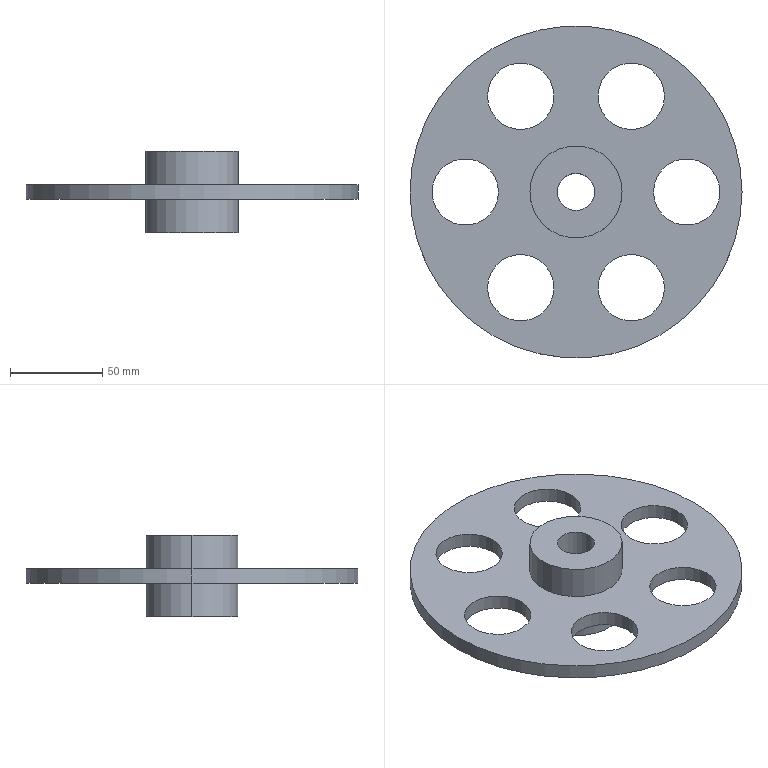Part | SolidWorks | features ICE 2, Extrusion 1 | 1 solid | 24 faces | box 180 x 180 x 44 mm | volume 211302 mm3 | cylinder 20 | plane 4 | commonest cylinder face diameters 36 x12 50 x4 20.2 x2 180 x2
STEP:
#1=CARTESIAN_POINT('',(12.,51.962,-4.));
#2=VERTEX_POINT('',#1);
#3=CARTESIAN_POINT('',(48.,51.962,-4.));
#4=VERTEX_POINT('',#3);
#5=CARTESIAN_POINT('',(30.,51.962,-4.));
#6=DIRECTION('',(0.,0.,1.));
#7=DIRECTION('',(1.,0.,0.));
#8=AXIS2_PLACEMENT_3D('',#5,#6,#7);
#9=CIRCLE('',#8,18.);
#10=EDGE_CURVE('',#2,#4,#9,.T.);
#11=ORIENTED_EDGE('',*,*,#10,.F.);
#12=CARTESIAN_POINT('',(12.,51.962,4.));
#13=VERTEX_POINT('',#12);
#14=CARTESIAN_POINT('',(12.,51.962,-30.));
#15=DIRECTION('',(0.,0.,1.));
#16=VECTOR('',#15,1000.);
#17=LINE('',#14,#16);
#18=EDGE_CURVE('',#2,#13,#17,.T.);
#19=ORIENTED_EDGE('',*,*,#18,.T.);
#20=CARTESIAN_POINT('',(48.,51.962,4.));
#21=VERTEX_POINT('',#20);
#22=CARTESIAN_POINT('',(30.,51.962,4.));
#23=DIRECTION('',(0.,0.,1.));
#24=DIRECTION('',(1.,0.,0.));
#25=AXIS2_PLACEMENT_3D('',#22,#23,#24);
#26=CIRCLE('',#25,18.);
#27=EDGE_CURVE('',#13,#21,#26,.T.);
#28=ORIENTED_EDGE('',*,*,#27,.T.);
#29=CARTESIAN_POINT('',(48.,51.962,-30.));
#30=DIRECTION('',(0.,0.,1.));
#31=VECTOR('',#30,1000.);
#32=LINE('',#29,#31);
#33=EDGE_CURVE('',#4,#21,#32,.T.);
#34=ORIENTED_EDGE('',*,*,#33,.F.);
#35=EDGE_LOOP('',(#11,#19,#28,#34));
#36=FACE_OUTER_BOUND('',#35,.T.);
#37=CARTESIAN_POINT('',(30.,51.962,-30.));
#38=DIRECTION('',(0.,0.,1.));
#39=DIRECTION('',(1.,0.,0.));
#40=AXIS2_PLACEMENT_3D('',#37,#38,#39);
#41=CYLINDRICAL_SURFACE('',#40,18.);
#42=ADVANCED_FACE('',(#36),#41,.F.);
#43=CARTESIAN_POINT('',(-48.,51.962,-4.));
#44=VERTEX_POINT('',#43);
#45=CARTESIAN_POINT('',(-12.,51.962,-4.));
#46=VERTEX_POINT('',#45);
#47=CARTESIAN_POINT('',(-30.,51.962,-4.));
#48=DIRECTION('',(0.,0.,1.));
#49=DIRECTION('',(1.,0.,0.));
#50=AXIS2_PLACEMENT_3D('',#47,#48,#49);
#51=CIRCLE('',#50,18.);
#52=EDGE_CURVE('',#44,#46,#51,.T.);
#53=ORIENTED_EDGE('',*,*,#52,.F.);
#54=CARTESIAN_POINT('',(-48.,51.962,4.));
#55=VERTEX_POINT('',#54);
#56=CARTESIAN_POINT('',(-48.,51.962,-30.));
#57=DIRECTION('',(0.,0.,1.));
#58=VECTOR('',#57,1000.);
#59=LINE('',#56,#58);
#60=EDGE_CURVE('',#44,#55,#59,.T.);
#61=ORIENTED_EDGE('',*,*,#60,.T.);
#62=CARTESIAN_POINT('',(-12.,51.962,4.));
#63=VERTEX_POINT('',#62);
#64=CARTESIAN_POINT('',(-30.,51.962,4.));
#65=DIRECTION('',(0.,0.,1.));
#66=DIRECTION('',(1.,0.,0.));
#67=AXIS2_PLACEMENT_3D('',#64,#65,#66);
#68=CIRCLE('',#67,18.);
#69=EDGE_CURVE('',#55,#63,#68,.T.);
#70=ORIENTED_EDGE('',*,*,#69,.T.);
#71=CARTESIAN_POINT('',(-12.,51.962,-30.));
#72=DIRECTION('',(0.,0.,1.));
#73=VECTOR('',#72,1000.);
#74=LINE('',#71,#73);
#75=EDGE_CURVE('',#46,#63,#74,.T.);
#76=ORIENTED_EDGE('',*,*,#75,.F.);
#77=EDGE_LOOP('',(#53,#61,#70,#76));
#78=FACE_OUTER_BOUND('',#77,.T.);
#79=CARTESIAN_POINT('',(-30.,51.962,-30.));
#80=DIRECTION('',(0.,0.,1.));
#81=DIRECTION('',(1.,0.,0.));
#82=AXIS2_PLACEMENT_3D('',#79,#80,#81);
#83=CYLINDRICAL_SURFACE('',#82,18.);
#84=ADVANCED_FACE('',(#78),#83,.F.);
#85=CARTESIAN_POINT('',(-78.,0.,-4.));
#86=VERTEX_POINT('',#85);
#87=CARTESIAN_POINT('',(-42.,0.,-4.));
#88=VERTEX_POINT('',#87);
#89=CARTESIAN_POINT('',(-60.,0.,-4.));
#90=DIRECTION('',(0.,0.,1.));
#91=DIRECTION('',(1.,0.,0.));
#92=AXIS2_PLACEMENT_3D('',#89,#90,#91);
#93=CIRCLE('',#92,18.);
#94=EDGE_CURVE('',#86,#88,#93,.T.);
#95=ORIENTED_EDGE('',*,*,#94,.F.);
#96=CARTESIAN_POINT('',(-78.,0.,4.));
#97=VERTEX_POINT('',#96);
#98=CARTESIAN_POINT('',(-78.,0.,-30.));
#99=DIRECTION('',(0.,0.,1.));
#100=VECTOR('',#99,1000.);
#101=LINE('',#98,#100);
#102=EDGE_CURVE('',#86,#97,#101,.T.);
#103=ORIENTED_EDGE('',*,*,#102,.T.);
#104=CARTESIAN_POINT('',(-42.,0.,4.));
#105=VERTEX_POINT('',#104);
#106=CARTESIAN_POINT('',(-60.,0.,4.));
#107=DIRECTION('',(0.,0.,1.));
#108=DIRECTION('',(1.,0.,0.));
#109=AXIS2_PLACEMENT_3D('',#106,#107,#108);
#110=CIRCLE('',#109,18.);
#111=EDGE_CURVE('',#97,#105,#110,.T.);
#112=ORIENTED_EDGE('',*,*,#111,.T.);
#113=CARTESIAN_POINT('',(-42.,0.,-30.));
#114=DIRECTION('',(0.,0.,1.));
#115=VECTOR('',#114,1000.);
#116=LINE('',#113,#115);
#117=EDGE_CURVE('',#88,#105,#116,.T.);
#118=ORIENTED_EDGE('',*,*,#117,.F.);
#119=EDGE_LOOP('',(#95,#103,#112,#118));
#120=FACE_OUTER_BOUND('',#119,.T.);
#121=CARTESIAN_POINT('',(-60.,0.,-30.));
#122=DIRECTION('',(0.,0.,1.));
#123=DIRECTION('',(1.,0.,0.));
#124=AXIS2_PLACEMENT_3D('',#121,#122,#123);
#125=CYLINDRICAL_SURFACE('',#124,18.);
#126=ADVANCED_FACE('',(#120),#125,.F.);
#127=CARTESIAN_POINT('',(-48.,-51.962,-4.));
#128=VERTEX_POINT('',#127);
#129=CARTESIAN_POINT('',(-12.,-51.962,-4.));
#130=VERTEX_POINT('',#129);
#131=CARTESIAN_POINT('',(-30.,-51.962,-4.));
#132=DIRECTION('',(0.,0.,1.));
#133=DIRECTION('',(1.,0.,0.));
#134=AXIS2_PLACEMENT_3D('',#131,#132,#133);
#135=CIRCLE('',#134,18.);
#136=EDGE_CURVE('',#128,#130,#135,.T.);
#137=ORIENTED_EDGE('',*,*,#136,.F.);
#138=CARTESIAN_POINT('',(-48.,-51.962,4.));
#139=VERTEX_POINT('',#138);
#140=CARTESIAN_POINT('',(-48.,-51.962,-30.));
#141=DIRECTION('',(0.,0.,1.));
#142=VECTOR('',#141,1000.);
#143=LINE('',#140,#142);
#144=EDGE_CURVE('',#128,#139,#143,.T.);
#145=ORIENTED_EDGE('',*,*,#144,.T.);
#146=CARTESIAN_POINT('',(-12.,-51.962,4.));
#147=VERTEX_POINT('',#146);
#148=CARTESIAN_POINT('',(-30.,-51.962,4.));
#149=DIRECTION('',(0.,0.,1.));
#150=DIRECTION('',(1.,0.,0.));
#151=AXIS2_PLACEMENT_3D('',#148,#149,#150);
#152=CIRCLE('',#151,18.);
#153=EDGE_CURVE('',#139,#147,#152,.T.);
#154=ORIENTED_EDGE('',*,*,#153,.T.);
#155=CARTESIAN_POINT('',(-12.,-51.962,-30.));
#156=DIRECTION('',(0.,0.,1.));
#157=VECTOR('',#156,1000.);
#158=LINE('',#155,#157);
#159=EDGE_CURVE('',#130,#147,#158,.T.);
#160=ORIENTED_EDGE('',*,*,#159,.F.);
#161=EDGE_LOOP('',(#137,#145,#154,#160));
#162=FACE_OUTER_BOUND('',#161,.T.);
#163=CARTESIAN_POINT('',(-30.,-51.962,-30.));
#164=DIRECTION('',(0.,0.,1.));
#165=DIRECTION('',(1.,0.,0.));
#166=AXIS2_PLACEMENT_3D('',#163,#164,#165);
#167=CYLINDRICAL_SURFACE('',#166,18.);
#168=ADVANCED_FACE('',(#162),#167,.F.);
#169=CARTESIAN_POINT('',(12.,-51.962,-4.));
#170=VERTEX_POINT('',#169);
#171=CARTESIAN_POINT('',(48.,-51.962,-4.));
#172=VERTEX_POINT('',#171);
#173=CARTESIAN_POINT('',(30.,-51.962,-4.));
#174=DIRECTION('',(0.,0.,1.));
#175=DIRECTION('',(1.,0.,0.));
#176=AXIS2_PLACEMENT_3D('',#173,#174,#175);
#177=CIRCLE('',#176,18.);
#178=EDGE_CURVE('',#170,#172,#177,.T.);
#179=ORIENTED_EDGE('',*,*,#178,.F.);
#180=CARTESIAN_POINT('',(12.,-51.962,4.));
#181=VERTEX_POINT('',#180);
#182=CARTESIAN_POINT('',(12.,-51.962,-30.));
#183=DIRECTION('',(0.,0.,1.));
#184=VECTOR('',#183,1000.);
#185=LINE('',#182,#184);
#186=EDGE_CURVE('',#170,#181,#185,.T.);
#187=ORIENTED_EDGE('',*,*,#186,.T.);
#188=CARTESIAN_POINT('',(48.,-51.962,4.));
#189=VERTEX_POINT('',#188);
#190=CARTESIAN_POINT('',(30.,-51.962,4.));
#191=DIRECTION('',(0.,0.,1.));
#192=DIRECTION('',(1.,0.,0.));
#193=AXIS2_PLACEMENT_3D('',#190,#191,#192);
#194=CIRCLE('',#193,18.);
#195=EDGE_CURVE('',#181,#189,#194,.T.);
#196=ORIENTED_EDGE('',*,*,#195,.T.);
#197=CARTESIAN_POINT('',(48.,-51.962,-30.));
#198=DIRECTION('',(0.,0.,1.));
#199=VECTOR('',#198,1000.);
#200=LINE('',#197,#199);
#201=EDGE_CURVE('',#172,#189,#200,.T.);
#202=ORIENTED_EDGE('',*,*,#201,.F.);
#203=EDGE_LOOP('',(#179,#187,#196,#202));
#204=FACE_OUTER_BOUND('',#203,.T.);
#205=CARTESIAN_POINT('',(30.,-51.962,-30.));
#206=DIRECTION('',(0.,0.,1.));
#207=DIRECTION('',(1.,0.,0.));
#208=AXIS2_PLACEMENT_3D('',#205,#206,#207);
#209=CYLINDRICAL_SURFACE('',#208,18.);
#210=ADVANCED_FACE('',(#204),#209,.F.);
#211=CARTESIAN_POINT('',(42.,0.,-4.));
#212=VERTEX_POINT('',#211);
#213=CARTESIAN_POINT('',(78.,0.,-4.));
#214=VERTEX_POINT('',#213);
#215=CARTESIAN_POINT('',(60.,0.,-4.));
#216=DIRECTION('',(0.,0.,1.));
#217=DIRECTION('',(1.,0.,0.));
#218=AXIS2_PLACEMENT_3D('',#215,#216,#217);
#219=CIRCLE('',#218,18.);
#220=EDGE_CURVE('',#212,#214,#219,.T.);
#221=ORIENTED_EDGE('',*,*,#220,.F.);
#222=CARTESIAN_POINT('',(42.,0.,4.));
#223=VERTEX_POINT('',#222);
#224=CARTESIAN_POINT('',(42.,0.,-30.));
#225=DIRECTION('',(0.,0.,1.));
#226=VECTOR('',#225,1000.);
#227=LINE('',#224,#226);
#228=EDGE_CURVE('',#212,#223,#227,.T.);
#229=ORIENTED_EDGE('',*,*,#228,.T.);
#230=CARTESIAN_POINT('',(78.,0.,4.));
#231=VERTEX_POINT('',#230);
#232=CARTESIAN_POINT('',(60.,0.,4.));
#233=DIRECTION('',(0.,0.,1.));
#234=DIRECTION('',(1.,0.,0.));
#235=AXIS2_PLACEMENT_3D('',#232,#233,#234);
#236=CIRCLE('',#235,18.);
#237=EDGE_CURVE('',#223,#231,#236,.T.);
#238=ORIENTED_EDGE('',*,*,#237,.T.);
#239=CARTESIAN_POINT('',(78.,0.,-30.));
#240=DIRECTION('',(0.,0.,1.));
#241=VECTOR('',#240,1000.);
#242=LINE('',#239,#241);
#243=EDGE_CURVE('',#214,#231,#242,.T.);
#244=ORIENTED_EDGE('',*,*,#243,.F.);
#245=EDGE_LOOP('',(#221,#229,#238,#244));
#246=FACE_OUTER_BOUND('',#245,.T.);
#247=CARTESIAN_POINT('',(60.,0.,-30.));
#248=DIRECTION('',(0.,0.,1.));
#249=DIRECTION('',(1.,0.,0.));
#250=AXIS2_PLACEMENT_3D('',#247,#248,#249);
#251=CYLINDRICAL_SURFACE('',#250,18.);
#252=ADVANCED_FACE('',(#246),#251,.F.);
#253=CARTESIAN_POINT('',(-10.1,0.,-22.));
#254=VERTEX_POINT('',#253);
#255=CARTESIAN_POINT('',(10.1,0.,-22.));
#256=VERTEX_POINT('',#255);
#257=CARTESIAN_POINT('',(0.,0.,-22.));
#258=DIRECTION('',(0.,0.,1.));
#259=DIRECTION('',(1.,0.,0.));
#260=AXIS2_PLACEMENT_3D('',#257,#258,#259);
#261=CIRCLE('',#260,10.1);
#262=EDGE_CURVE('',#254,#256,#261,.T.);
#263=ORIENTED_EDGE('',*,*,#262,.F.);
#264=CARTESIAN_POINT('',(-10.1,0.,22.));
#265=VERTEX_POINT('',#264);
#266=CARTESIAN_POINT('',(-10.1,0.,-4.));
#267=DIRECTION('',(0.,0.,1.));
#268=VECTOR('',#267,1000.);
#269=LINE('',#266,#268);
#270=EDGE_CURVE('',#254,#265,#269,.T.);
#271=ORIENTED_EDGE('',*,*,#270,.T.);
#272=CARTESIAN_POINT('',(10.1,0.,22.));
#273=VERTEX_POINT('',#272);
#274=CARTESIAN_POINT('',(0.,0.,22.));
#275=DIRECTION('',(0.,0.,1.));
#276=DIRECTION('',(1.,0.,0.));
#277=AXIS2_PLACEMENT_3D('',#274,#275,#276);
#278=CIRCLE('',#277,10.1);
#279=EDGE_CURVE('',#265,#273,#278,.T.);
#280=ORIENTED_EDGE('',*,*,#279,.T.);
#281=CARTESIAN_POINT('',(10.1,0.,-4.));
#282=DIRECTION('',(0.,0.,1.));
#283=VECTOR('',#282,1000.);
#284=LINE('',#281,#283);
#285=EDGE_CURVE('',#256,#273,#284,.T.);
#286=ORIENTED_EDGE('',*,*,#285,.F.);
#287=EDGE_LOOP('',(#263,#271,#280,#286));
#288=FACE_OUTER_BOUND('',#287,.T.);
#289=CARTESIAN_POINT('',(0.,0.,-4.));
#290=DIRECTION('',(0.,0.,1.));
#291=DIRECTION('',(1.,0.,0.));
#292=AXIS2_PLACEMENT_3D('',#289,#290,#291);
#293=CYLINDRICAL_SURFACE('',#292,10.1);
#294=ADVANCED_FACE('',(#288),#293,.F.);
#295=CARTESIAN_POINT('',(25.,0.,-22.));
#296=VERTEX_POINT('',#295);
#297=CARTESIAN_POINT('',(-25.,0.,-22.));
#298=VERTEX_POINT('',#297);
#299=CARTESIAN_POINT('',(0.,0.,-22.));
#300=DIRECTION('',(0.,0.,1.));
#301=DIRECTION('',(1.,0.,0.));
#302=AXIS2_PLACEMENT_3D('',#299,#300,#301);
#303=CIRCLE('',#302,25.);
#304=EDGE_CURVE('',#296,#298,#303,.T.);
#305=ORIENTED_EDGE('',*,*,#304,.T.);
#306=CARTESIAN_POINT('',(-25.,0.,-4.));
#307=VERTEX_POINT('',#306);
#308=CARTESIAN_POINT('',(-25.,0.,-22.));
#309=DIRECTION('',(0.,0.,1.));
#310=VECTOR('',#309,1000.);
#311=LINE('',#308,#310);
#312=EDGE_CURVE('',#298,#307,#311,.T.);
#313=ORIENTED_EDGE('',*,*,#312,.T.);
#314=CARTESIAN_POINT('',(25.,0.,-4.));
#315=VERTEX_POINT('',#314);
#316=CARTESIAN_POINT('',(0.,0.,-4.));
#317=DIRECTION('',(0.,0.,1.));
#318=DIRECTION('',(1.,0.,0.));
#319=AXIS2_PLACEMENT_3D('',#316,#317,#318);
#320=CIRCLE('',#319,25.);
#321=EDGE_CURVE('',#315,#307,#320,.T.);
#322=ORIENTED_EDGE('',*,*,#321,.F.);
#323=CARTESIAN_POINT('',(25.,0.,-22.));
#324=DIRECTION('',(0.,0.,1.));
#325=VECTOR('',#324,1000.);
#326=LINE('',#323,#325);
#327=EDGE_CURVE('',#296,#315,#326,.T.);
#328=ORIENTED_EDGE('',*,*,#327,.F.);
#329=EDGE_LOOP('',(#305,#313,#322,#328));
#330=FACE_OUTER_BOUND('',#329,.T.);
#331=CARTESIAN_POINT('',(0.,0.,-22.));
#332=DIRECTION('',(0.,0.,1.));
#333=DIRECTION('',(1.,0.,0.));
#334=AXIS2_PLACEMENT_3D('',#331,#332,#333);
#335=CYLINDRICAL_SURFACE('',#334,25.);
#336=ADVANCED_FACE('',(#330),#335,.T.);
#337=CARTESIAN_POINT('',(25.,0.,4.));
#338=VERTEX_POINT('',#337);
#339=CARTESIAN_POINT('',(-25.,0.,4.));
#340=VERTEX_POINT('',#339);
#341=CARTESIAN_POINT('',(0.,0.,4.));
#342=DIRECTION('',(0.,0.,1.));
#343=DIRECTION('',(1.,0.,0.));
#344=AXIS2_PLACEMENT_3D('',#341,#342,#343);
#345=CIRCLE('',#344,25.);
#346=EDGE_CURVE('',#338,#340,#345,.T.);
#347=ORIENTED_EDGE('',*,*,#346,.T.);
#348=CARTESIAN_POINT('',(-25.,0.,22.));
#349=VERTEX_POINT('',#348);
#350=CARTESIAN_POINT('',(-25.,0.,-22.));
#351=DIRECTION('',(0.,0.,1.));
#352=VECTOR('',#351,1000.);
#353=LINE('',#350,#352);
#354=EDGE_CURVE('',#340,#349,#353,.T.);
#355=ORIENTED_EDGE('',*,*,#354,.T.);
#356=CARTESIAN_POINT('',(25.,0.,22.));
#357=VERTEX_POINT('',#356);
#358=CARTESIAN_POINT('',(0.,0.,22.));
#359=DIRECTION('',(0.,0.,1.));
#360=DIRECTION('',(1.,0.,0.));
#361=AXIS2_PLACEMENT_3D('',#358,#359,#360);
#362=CIRCLE('',#361,25.);
#363=EDGE_CURVE('',#357,#349,#362,.T.);
#364=ORIENTED_EDGE('',*,*,#363,.F.);
#365=CARTESIAN_POINT('',(25.,0.,-22.));
#366=DIRECTION('',(0.,0.,1.));
#367=VECTOR('',#366,1000.);
#368=LINE('',#365,#367);
#369=EDGE_CURVE('',#338,#357,#368,.T.);
#370=ORIENTED_EDGE('',*,*,#369,.F.);
#371=EDGE_LOOP('',(#347,#355,#364,#370));
#372=FACE_OUTER_BOUND('',#371,.T.);
#373=CARTESIAN_POINT('',(0.,0.,-22.));
#374=DIRECTION('',(0.,0.,1.));
#375=DIRECTION('',(1.,0.,0.));
#376=AXIS2_PLACEMENT_3D('',#373,#374,#375);
#377=CYLINDRICAL_SURFACE('',#376,25.);
#378=ADVANCED_FACE('',(#372),#377,.T.);
#379=CARTESIAN_POINT('',(90.,0.,-4.));
#380=VERTEX_POINT('',#379);
#381=CARTESIAN_POINT('',(-90.,0.,-4.));
#382=VERTEX_POINT('',#381);
#383=CARTESIAN_POINT('',(0.,0.,-4.));
#384=DIRECTION('',(0.,0.,1.));
#385=DIRECTION('',(1.,0.,0.));
#386=AXIS2_PLACEMENT_3D('',#383,#384,#385);
#387=CIRCLE('',#386,90.);
#388=EDGE_CURVE('',#380,#382,#387,.T.);
#389=ORIENTED_EDGE('',*,*,#388,.T.);
#390=CARTESIAN_POINT('',(-90.,0.,4.));
#391=VERTEX_POINT('',#390);
#392=CARTESIAN_POINT('',(-90.,0.,-4.));
#393=DIRECTION('',(0.,0.,1.));
#394=VECTOR('',#393,1000.);
#395=LINE('',#392,#394);
#396=EDGE_CURVE('',#382,#391,#395,.T.);
#397=ORIENTED_EDGE('',*,*,#396,.T.);
#398=CARTESIAN_POINT('',(90.,0.,4.));
#399=VERTEX_POINT('',#398);
#400=CARTESIAN_POINT('',(0.,0.,4.));
#401=DIRECTION('',(0.,0.,1.));
#402=DIRECTION('',(1.,0.,0.));
#403=AXIS2_PLACEMENT_3D('',#400,#401,#402);
#404=CIRCLE('',#403,90.);
#405=EDGE_CURVE('',#399,#391,#404,.T.);
#406=ORIENTED_EDGE('',*,*,#405,.F.);
#407=CARTESIAN_POINT('',(90.,0.,-4.));
#408=DIRECTION('',(0.,0.,1.));
#409=VECTOR('',#408,1000.);
#410=LINE('',#407,#409);
#411=EDGE_CURVE('',#380,#399,#410,.T.);
#412=ORIENTED_EDGE('',*,*,#411,.F.);
#413=EDGE_LOOP('',(#389,#397,#406,#412));
#414=FACE_OUTER_BOUND('',#413,.T.);
#415=CARTESIAN_POINT('',(0.,0.,-4.));
#416=DIRECTION('',(0.,0.,1.));
#417=DIRECTION('',(1.,0.,0.));
#418=AXIS2_PLACEMENT_3D('',#415,#416,#417);
#419=CYLINDRICAL_SURFACE('',#418,90.);
#420=ADVANCED_FACE('',(#414),#419,.T.);
#421=ORIENTED_EDGE('',*,*,#396,.F.);
#422=CARTESIAN_POINT('',(0.,0.,-4.));
#423=DIRECTION('',(0.,0.,1.));
#424=DIRECTION('',(1.,0.,0.));
#425=AXIS2_PLACEMENT_3D('',#422,#423,#424);
#426=CIRCLE('',#425,90.);
#427=EDGE_CURVE('',#382,#380,#426,.T.);
#428=ORIENTED_EDGE('',*,*,#427,.T.);
#429=ORIENTED_EDGE('',*,*,#411,.T.);
#430=CARTESIAN_POINT('',(0.,0.,4.));
#431=DIRECTION('',(0.,0.,1.));
#432=DIRECTION('',(1.,0.,0.));
#433=AXIS2_PLACEMENT_3D('',#430,#431,#432);
#434=CIRCLE('',#433,90.);
#435=EDGE_CURVE('',#391,#399,#434,.T.);
#436=ORIENTED_EDGE('',*,*,#435,.F.);
#437=EDGE_LOOP('',(#421,#428,#429,#436));
#438=FACE_OUTER_BOUND('',#437,.T.);
#439=CARTESIAN_POINT('',(0.,0.,-4.));
#440=DIRECTION('',(0.,0.,1.));
#441=DIRECTION('',(1.,0.,0.));
#442=AXIS2_PLACEMENT_3D('',#439,#440,#441);
#443=CYLINDRICAL_SURFACE('',#442,90.);
#444=ADVANCED_FACE('',(#438),#443,.T.);
#445=CARTESIAN_POINT('',(30.,51.962,-4.));
#446=DIRECTION('',(0.,0.,1.));
#447=DIRECTION('',(1.,0.,0.));
#448=AXIS2_PLACEMENT_3D('',#445,#446,#447);
#449=CIRCLE('',#448,18.);
#450=EDGE_CURVE('',#4,#2,#449,.T.);
#451=ORIENTED_EDGE('',*,*,#450,.T.);
#452=ORIENTED_EDGE('',*,*,#10,.T.);
#453=EDGE_LOOP('',(#451,#452));
#454=FACE_BOUND('',#453,.T.);
#455=CARTESIAN_POINT('',(-30.,51.962,-4.));
#456=DIRECTION('',(0.,0.,1.));
#457=DIRECTION('',(1.,0.,0.));
#458=AXIS2_PLACEMENT_3D('',#455,#456,#457);
#459=CIRCLE('',#458,18.);
#460=EDGE_CURVE('',#46,#44,#459,.T.);
#461=ORIENTED_EDGE('',*,*,#460,.T.);
#462=ORIENTED_EDGE('',*,*,#52,.T.);
#463=EDGE_LOOP('',(#461,#462));
#464=FACE_BOUND('',#463,.T.);
#465=CARTESIAN_POINT('',(-60.,0.,-4.));
#466=DIRECTION('',(0.,0.,1.));
#467=DIRECTION('',(1.,0.,0.));
#468=AXIS2_PLACEMENT_3D('',#465,#466,#467);
#469=CIRCLE('',#468,18.);
#470=EDGE_CURVE('',#88,#86,#469,.T.);
#471=ORIENTED_EDGE('',*,*,#470,.T.);
#472=ORIENTED_EDGE('',*,*,#94,.T.);
#473=EDGE_LOOP('',(#471,#472));
#474=FACE_BOUND('',#473,.T.);
#475=CARTESIAN_POINT('',(-30.,-51.962,-4.));
#476=DIRECTION('',(0.,0.,1.));
#477=DIRECTION('',(1.,0.,0.));
#478=AXIS2_PLACEMENT_3D('',#475,#476,#477);
#479=CIRCLE('',#478,18.);
#480=EDGE_CURVE('',#130,#128,#479,.T.);
#481=ORIENTED_EDGE('',*,*,#480,.T.);
#482=ORIENTED_EDGE('',*,*,#136,.T.);
#483=EDGE_LOOP('',(#481,#482));
#484=FACE_BOUND('',#483,.T.);
#485=CARTESIAN_POINT('',(30.,-51.962,-4.));
#486=DIRECTION('',(0.,0.,1.));
#487=DIRECTION('',(1.,0.,0.));
#488=AXIS2_PLACEMENT_3D('',#485,#486,#487);
#489=CIRCLE('',#488,18.);
#490=EDGE_CURVE('',#172,#170,#489,.T.);
#491=ORIENTED_EDGE('',*,*,#490,.T.);
#492=ORIENTED_EDGE('',*,*,#178,.T.);
#493=EDGE_LOOP('',(#491,#492));
#494=FACE_BOUND('',#493,.T.);
#495=CARTESIAN_POINT('',(60.,0.,-4.));
#496=DIRECTION('',(0.,0.,1.));
#497=DIRECTION('',(1.,0.,0.));
#498=AXIS2_PLACEMENT_3D('',#495,#496,#497);
#499=CIRCLE('',#498,18.);
#500=EDGE_CURVE('',#214,#212,#499,.T.);
#501=ORIENTED_EDGE('',*,*,#500,.T.);
#502=ORIENTED_EDGE('',*,*,#220,.T.);
#503=EDGE_LOOP('',(#501,#502));
#504=FACE_BOUND('',#503,.T.);
#505=ORIENTED_EDGE('',*,*,#321,.T.);
#506=CARTESIAN_POINT('',(0.,0.,-4.));
#507=DIRECTION('',(0.,0.,1.));
#508=DIRECTION('',(1.,0.,0.));
#509=AXIS2_PLACEMENT_3D('',#506,#507,#508);
#510=CIRCLE('',#509,25.);
#511=EDGE_CURVE('',#307,#315,#510,.T.);
#512=ORIENTED_EDGE('',*,*,#511,.T.);
#513=EDGE_LOOP('',(#505,#512));
#514=FACE_BOUND('',#513,.T.);
#515=ORIENTED_EDGE('',*,*,#388,.F.);
#516=ORIENTED_EDGE('',*,*,#427,.F.);
#517=EDGE_LOOP('',(#515,#516));
#518=FACE_OUTER_BOUND('',#517,.T.);
#519=CARTESIAN_POINT('',(0.,0.,-4.));
#520=DIRECTION('',(0.,0.,1.));
#521=DIRECTION('',(1.,0.,0.));
#522=AXIS2_PLACEMENT_3D('',#519,#520,#521);
#523=PLANE('',#522);
#524=ADVANCED_FACE('',(#454,#464,#474,#484,#494,#504,#514,#518),#523,.F.);
#525=CARTESIAN_POINT('',(30.,51.962,4.));
#526=DIRECTION('',(0.,0.,1.));
#527=DIRECTION('',(1.,0.,0.));
#528=AXIS2_PLACEMENT_3D('',#525,#526,#527);
#529=CIRCLE('',#528,18.);
#530=EDGE_CURVE('',#21,#13,#529,.T.);
#531=ORIENTED_EDGE('',*,*,#530,.F.);
#532=ORIENTED_EDGE('',*,*,#27,.F.);
#533=EDGE_LOOP('',(#531,#532));
#534=FACE_BOUND('',#533,.T.);
#535=CARTESIAN_POINT('',(-30.,51.962,4.));
#536=DIRECTION('',(0.,0.,1.));
#537=DIRECTION('',(1.,0.,0.));
#538=AXIS2_PLACEMENT_3D('',#535,#536,#537);
#539=CIRCLE('',#538,18.);
#540=EDGE_CURVE('',#63,#55,#539,.T.);
#541=ORIENTED_EDGE('',*,*,#540,.F.);
#542=ORIENTED_EDGE('',*,*,#69,.F.);
#543=EDGE_LOOP('',(#541,#542));
#544=FACE_BOUND('',#543,.T.);
#545=CARTESIAN_POINT('',(-60.,0.,4.));
#546=DIRECTION('',(0.,0.,1.));
#547=DIRECTION('',(1.,0.,0.));
#548=AXIS2_PLACEMENT_3D('',#545,#546,#547);
#549=CIRCLE('',#548,18.);
#550=EDGE_CURVE('',#105,#97,#549,.T.);
#551=ORIENTED_EDGE('',*,*,#550,.F.);
#552=ORIENTED_EDGE('',*,*,#111,.F.);
#553=EDGE_LOOP('',(#551,#552));
#554=FACE_BOUND('',#553,.T.);
#555=CARTESIAN_POINT('',(-30.,-51.962,4.));
#556=DIRECTION('',(0.,0.,1.));
#557=DIRECTION('',(1.,0.,0.));
#558=AXIS2_PLACEMENT_3D('',#555,#556,#557);
#559=CIRCLE('',#558,18.);
#560=EDGE_CURVE('',#147,#139,#559,.T.);
#561=ORIENTED_EDGE('',*,*,#560,.F.);
#562=ORIENTED_EDGE('',*,*,#153,.F.);
#563=EDGE_LOOP('',(#561,#562));
#564=FACE_BOUND('',#563,.T.);
#565=CARTESIAN_POINT('',(30.,-51.962,4.));
#566=DIRECTION('',(0.,0.,1.));
#567=DIRECTION('',(1.,0.,0.));
#568=AXIS2_PLACEMENT_3D('',#565,#566,#567);
#569=CIRCLE('',#568,18.);
#570=EDGE_CURVE('',#189,#181,#569,.T.);
#571=ORIENTED_EDGE('',*,*,#570,.F.);
#572=ORIENTED_EDGE('',*,*,#195,.F.);
#573=EDGE_LOOP('',(#571,#572));
#574=FACE_BOUND('',#573,.T.);
#575=CARTESIAN_POINT('',(60.,0.,4.));
#576=DIRECTION('',(0.,0.,1.));
#577=DIRECTION('',(1.,0.,0.));
#578=AXIS2_PLACEMENT_3D('',#575,#576,#577);
#579=CIRCLE('',#578,18.);
#580=EDGE_CURVE('',#231,#223,#579,.T.);
#581=ORIENTED_EDGE('',*,*,#580,.F.);
#582=ORIENTED_EDGE('',*,*,#237,.F.);
#583=EDGE_LOOP('',(#581,#582));
#584=FACE_BOUND('',#583,.T.);
#585=ORIENTED_EDGE('',*,*,#346,.F.);
#586=CARTESIAN_POINT('',(0.,0.,4.));
#587=DIRECTION('',(0.,0.,1.));
#588=DIRECTION('',(1.,0.,0.));
#589=AXIS2_PLACEMENT_3D('',#586,#587,#588);
#590=CIRCLE('',#589,25.);
#591=EDGE_CURVE('',#340,#338,#590,.T.);
#592=ORIENTED_EDGE('',*,*,#591,.F.);
#593=EDGE_LOOP('',(#585,#592));
#594=FACE_BOUND('',#593,.T.);
#595=ORIENTED_EDGE('',*,*,#405,.T.);
#596=ORIENTED_EDGE('',*,*,#435,.T.);
#597=EDGE_LOOP('',(#595,#596));
#598=FACE_OUTER_BOUND('',#597,.T.);
#599=CARTESIAN_POINT('',(0.,0.,4.));
#600=DIRECTION('',(0.,0.,1.));
#601=DIRECTION('',(1.,0.,0.));
#602=AXIS2_PLACEMENT_3D('',#599,#600,#601);
#603=PLANE('',#602);
#604=ADVANCED_FACE('',(#534,#544,#554,#564,#574,#584,#594,#598),#603,.T.);
#605=ORIENTED_EDGE('',*,*,#354,.F.);
#606=ORIENTED_EDGE('',*,*,#591,.T.);
#607=ORIENTED_EDGE('',*,*,#369,.T.);
#608=CARTESIAN_POINT('',(0.,0.,22.));
#609=DIRECTION('',(0.,0.,1.));
#610=DIRECTION('',(1.,0.,0.));
#611=AXIS2_PLACEMENT_3D('',#608,#609,#610);
#612=CIRCLE('',#611,25.);
#613=EDGE_CURVE('',#349,#357,#612,.T.);
#614=ORIENTED_EDGE('',*,*,#613,.F.);
#615=EDGE_LOOP('',(#605,#606,#607,#614));
#616=FACE_OUTER_BOUND('',#615,.T.);
#617=CARTESIAN_POINT('',(0.,0.,-22.));
#618=DIRECTION('',(0.,0.,1.));
#619=DIRECTION('',(1.,0.,0.));
#620=AXIS2_PLACEMENT_3D('',#617,#618,#619);
#621=CYLINDRICAL_SURFACE('',#620,25.);
#622=ADVANCED_FACE('',(#616),#621,.T.);
#623=CARTESIAN_POINT('',(0.,0.,22.));
#624=DIRECTION('',(0.,0.,1.));
#625=DIRECTION('',(1.,0.,0.));
#626=AXIS2_PLACEMENT_3D('',#623,#624,#625);
#627=CIRCLE('',#626,10.1);
#628=EDGE_CURVE('',#273,#265,#627,.T.);
#629=ORIENTED_EDGE('',*,*,#628,.F.);
#630=ORIENTED_EDGE('',*,*,#279,.F.);
#631=EDGE_LOOP('',(#629,#630));
#632=FACE_BOUND('',#631,.T.);
#633=ORIENTED_EDGE('',*,*,#363,.T.);
#634=ORIENTED_EDGE('',*,*,#613,.T.);
#635=EDGE_LOOP('',(#633,#634));
#636=FACE_OUTER_BOUND('',#635,.T.);
#637=CARTESIAN_POINT('',(0.,0.,22.));
#638=DIRECTION('',(0.,0.,1.));
#639=DIRECTION('',(1.,0.,0.));
#640=AXIS2_PLACEMENT_3D('',#637,#638,#639);
#641=PLANE('',#640);
#642=ADVANCED_FACE('',(#632,#636),#641,.T.);
#643=ORIENTED_EDGE('',*,*,#312,.F.);
#644=CARTESIAN_POINT('',(0.,0.,-22.));
#645=DIRECTION('',(0.,0.,1.));
#646=DIRECTION('',(1.,0.,0.));
#647=AXIS2_PLACEMENT_3D('',#644,#645,#646);
#648=CIRCLE('',#647,25.);
#649=EDGE_CURVE('',#298,#296,#648,.T.);
#650=ORIENTED_EDGE('',*,*,#649,.T.);
#651=ORIENTED_EDGE('',*,*,#327,.T.);
#652=ORIENTED_EDGE('',*,*,#511,.F.);
#653=EDGE_LOOP('',(#643,#650,#651,#652));
#654=FACE_OUTER_BOUND('',#653,.T.);
#655=CARTESIAN_POINT('',(0.,0.,-22.));
#656=DIRECTION('',(0.,0.,1.));
#657=DIRECTION('',(1.,0.,0.));
#658=AXIS2_PLACEMENT_3D('',#655,#656,#657);
#659=CYLINDRICAL_SURFACE('',#658,25.);
#660=ADVANCED_FACE('',(#654),#659,.T.);
#661=CARTESIAN_POINT('',(0.,0.,-22.));
#662=DIRECTION('',(0.,0.,1.));
#663=DIRECTION('',(1.,0.,0.));
#664=AXIS2_PLACEMENT_3D('',#661,#662,#663);
#665=CIRCLE('',#664,10.1);
#666=EDGE_CURVE('',#256,#254,#665,.T.);
#667=ORIENTED_EDGE('',*,*,#666,.T.);
#668=ORIENTED_EDGE('',*,*,#262,.T.);
#669=EDGE_LOOP('',(#667,#668));
#670=FACE_BOUND('',#669,.T.);
#671=ORIENTED_EDGE('',*,*,#304,.F.);
#672=ORIENTED_EDGE('',*,*,#649,.F.);
#673=EDGE_LOOP('',(#671,#672));
#674=FACE_OUTER_BOUND('',#673,.T.);
#675=CARTESIAN_POINT('',(0.,0.,-22.));
#676=DIRECTION('',(0.,0.,1.));
#677=DIRECTION('',(1.,0.,0.));
#678=AXIS2_PLACEMENT_3D('',#675,#676,#677);
#679=PLANE('',#678);
#680=ADVANCED_FACE('',(#670,#674),#679,.F.);
#681=ORIENTED_EDGE('',*,*,#270,.F.);
#682=ORIENTED_EDGE('',*,*,#666,.F.);
#683=ORIENTED_EDGE('',*,*,#285,.T.);
#684=ORIENTED_EDGE('',*,*,#628,.T.);
#685=EDGE_LOOP('',(#681,#682,#683,#684));
#686=FACE_OUTER_BOUND('',#685,.T.);
#687=CARTESIAN_POINT('',(0.,0.,-4.));
#688=DIRECTION('',(0.,0.,1.));
#689=DIRECTION('',(1.,0.,0.));
#690=AXIS2_PLACEMENT_3D('',#687,#688,#689);
#691=CYLINDRICAL_SURFACE('',#690,10.1);
#692=ADVANCED_FACE('',(#686),#691,.F.);
#693=ORIENTED_EDGE('',*,*,#228,.F.);
#694=ORIENTED_EDGE('',*,*,#500,.F.);
#695=ORIENTED_EDGE('',*,*,#243,.T.);
#696=ORIENTED_EDGE('',*,*,#580,.T.);
#697=EDGE_LOOP('',(#693,#694,#695,#696));
#698=FACE_OUTER_BOUND('',#697,.T.);
#699=CARTESIAN_POINT('',(60.,0.,-30.));
#700=DIRECTION('',(0.,0.,1.));
#701=DIRECTION('',(1.,0.,0.));
#702=AXIS2_PLACEMENT_3D('',#699,#700,#701);
#703=CYLINDRICAL_SURFACE('',#702,18.);
#704=ADVANCED_FACE('',(#698),#703,.F.);
#705=ORIENTED_EDGE('',*,*,#186,.F.);
#706=ORIENTED_EDGE('',*,*,#490,.F.);
#707=ORIENTED_EDGE('',*,*,#201,.T.);
#708=ORIENTED_EDGE('',*,*,#570,.T.);
#709=EDGE_LOOP('',(#705,#706,#707,#708));
#710=FACE_OUTER_BOUND('',#709,.T.);
#711=CARTESIAN_POINT('',(30.,-51.962,-30.));
#712=DIRECTION('',(0.,0.,1.));
#713=DIRECTION('',(1.,0.,0.));
#714=AXIS2_PLACEMENT_3D('',#711,#712,#713);
#715=CYLINDRICAL_SURFACE('',#714,18.);
#716=ADVANCED_FACE('',(#710),#715,.F.);
#717=ORIENTED_EDGE('',*,*,#144,.F.);
#718=ORIENTED_EDGE('',*,*,#480,.F.);
#719=ORIENTED_EDGE('',*,*,#159,.T.);
#720=ORIENTED_EDGE('',*,*,#560,.T.);
#721=EDGE_LOOP('',(#717,#718,#719,#720));
#722=FACE_OUTER_BOUND('',#721,.T.);
#723=CARTESIAN_POINT('',(-30.,-51.962,-30.));
#724=DIRECTION('',(0.,0.,1.));
#725=DIRECTION('',(1.,0.,0.));
#726=AXIS2_PLACEMENT_3D('',#723,#724,#725);
#727=CYLINDRICAL_SURFACE('',#726,18.);
#728=ADVANCED_FACE('',(#722),#727,.F.);
#729=ORIENTED_EDGE('',*,*,#102,.F.);
#730=ORIENTED_EDGE('',*,*,#470,.F.);
#731=ORIENTED_EDGE('',*,*,#117,.T.);
#732=ORIENTED_EDGE('',*,*,#550,.T.);
#733=EDGE_LOOP('',(#729,#730,#731,#732));
#734=FACE_OUTER_BOUND('',#733,.T.);
#735=CARTESIAN_POINT('',(-60.,0.,-30.));
#736=DIRECTION('',(0.,0.,1.));
#737=DIRECTION('',(1.,0.,0.));
#738=AXIS2_PLACEMENT_3D('',#735,#736,#737);
#739=CYLINDRICAL_SURFACE('',#738,18.);
#740=ADVANCED_FACE('',(#734),#739,.F.);
#741=ORIENTED_EDGE('',*,*,#60,.F.);
#742=ORIENTED_EDGE('',*,*,#460,.F.);
#743=ORIENTED_EDGE('',*,*,#75,.T.);
#744=ORIENTED_EDGE('',*,*,#540,.T.);
#745=EDGE_LOOP('',(#741,#742,#743,#744));
#746=FACE_OUTER_BOUND('',#745,.T.);
#747=CARTESIAN_POINT('',(-30.,51.962,-30.));
#748=DIRECTION('',(0.,0.,1.));
#749=DIRECTION('',(1.,0.,0.));
#750=AXIS2_PLACEMENT_3D('',#747,#748,#749);
#751=CYLINDRICAL_SURFACE('',#750,18.);
#752=ADVANCED_FACE('',(#746),#751,.F.);
#753=ORIENTED_EDGE('',*,*,#18,.F.);
#754=ORIENTED_EDGE('',*,*,#450,.F.);
#755=ORIENTED_EDGE('',*,*,#33,.T.);
#756=ORIENTED_EDGE('',*,*,#530,.T.);
#757=EDGE_LOOP('',(#753,#754,#755,#756));
#758=FACE_OUTER_BOUND('',#757,.T.);
#759=CARTESIAN_POINT('',(30.,51.962,-30.));
#760=DIRECTION('',(0.,0.,1.));
#761=DIRECTION('',(1.,0.,0.));
#762=AXIS2_PLACEMENT_3D('',#759,#760,#761);
#763=CYLINDRICAL_SURFACE('',#762,18.);
#764=ADVANCED_FACE('',(#758),#763,.F.);
#765=CLOSED_SHELL('',(#42,#84,#126,#168,#210,#252,#294,#336,#378,#420,#444,#524,#604,#622,#642,#660,#680,#692,#704,#716,#728,#740,#752,#764));
#766=MANIFOLD_SOLID_BREP('',#765);
#767=CARTESIAN_POINT('',(0.,0.,0.));
#768=DIRECTION('',(0.,0.,1.));
#769=DIRECTION('',(1.,0.,0.));
#770=AXIS2_PLACEMENT_3D('',#767,#768,#769);
#771=(LENGTH_UNIT()NAMED_UNIT(*)SI_UNIT(.MILLI.,.METRE.));
#772=UNCERTAINTY_MEASURE_WITH_UNIT(LENGTH_MEASURE(0.00001),#771,'','');
#773=(NAMED_UNIT(*)PLANE_ANGLE_UNIT()SI_UNIT($,.RADIAN.));
#774=(NAMED_UNIT(*)SI_UNIT($,.STERADIAN.)SOLID_ANGLE_UNIT());
#775=(GEOMETRIC_REPRESENTATION_CONTEXT(3)GLOBAL_UNCERTAINTY_ASSIGNED_CONTEXT((#772))GLOBAL_UNIT_ASSIGNED_CONTEXT((#771,#773,#774))REPRESENTATION_CONTEXT('',''));
#776=ADVANCED_BREP_SHAPE_REPRESENTATION('',(#766,#770),#775);